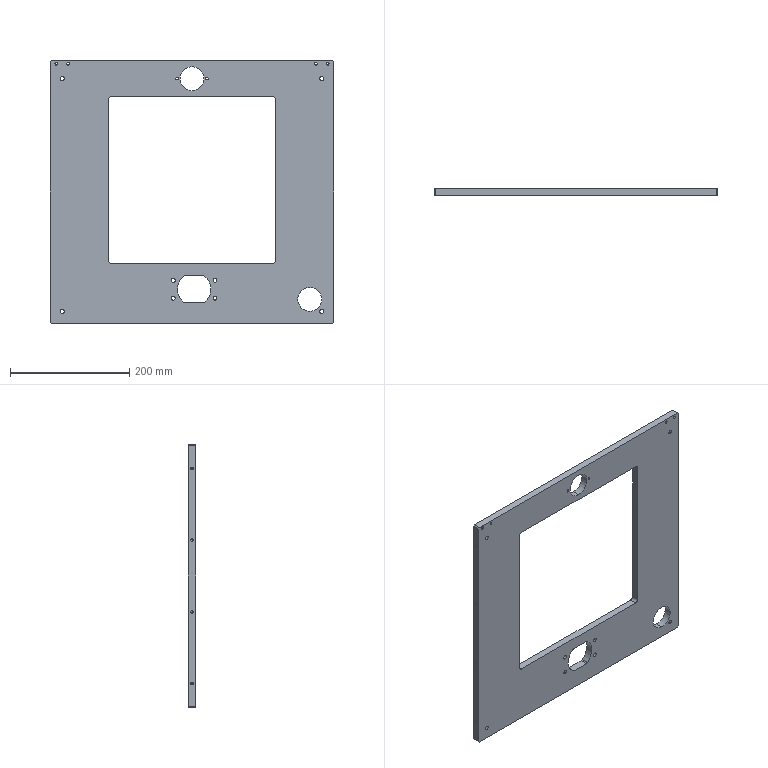Part | SolidWorks | features HoleWzd 6, ICE 3, Fillet 2, Chamfer 1, Cut 1, Extrusion 1, MirrorPattern 1 | 1 solid | 130 faces | box 475 x 12 x 440 mm | volume 1500689 mm3 | cylinder 82 | cone 24 | plane 24 | commonest cylinder face diameters 4.2 x28 6.6 x16 11 x16 4.5 x8 10 x8 40 x4